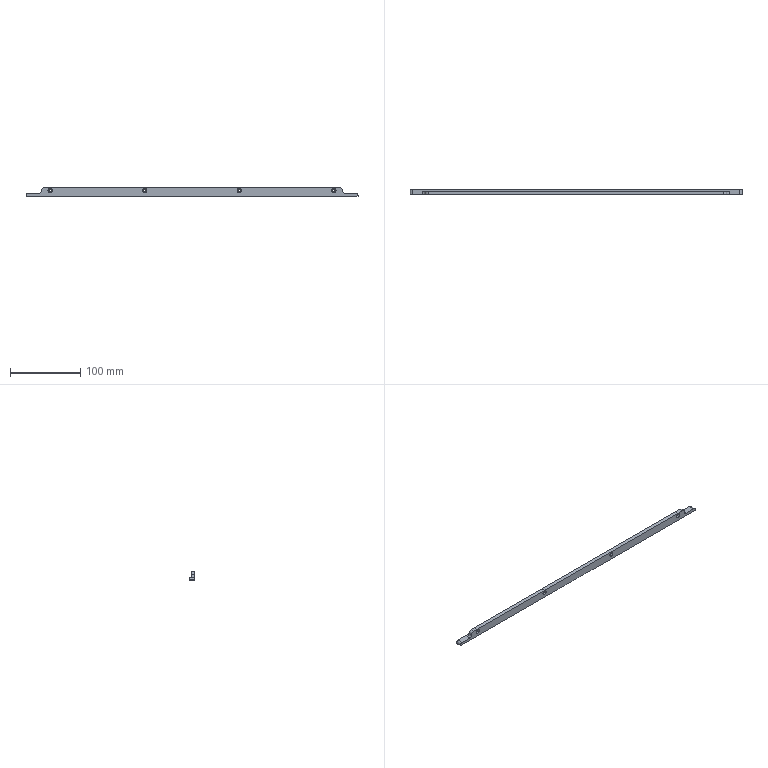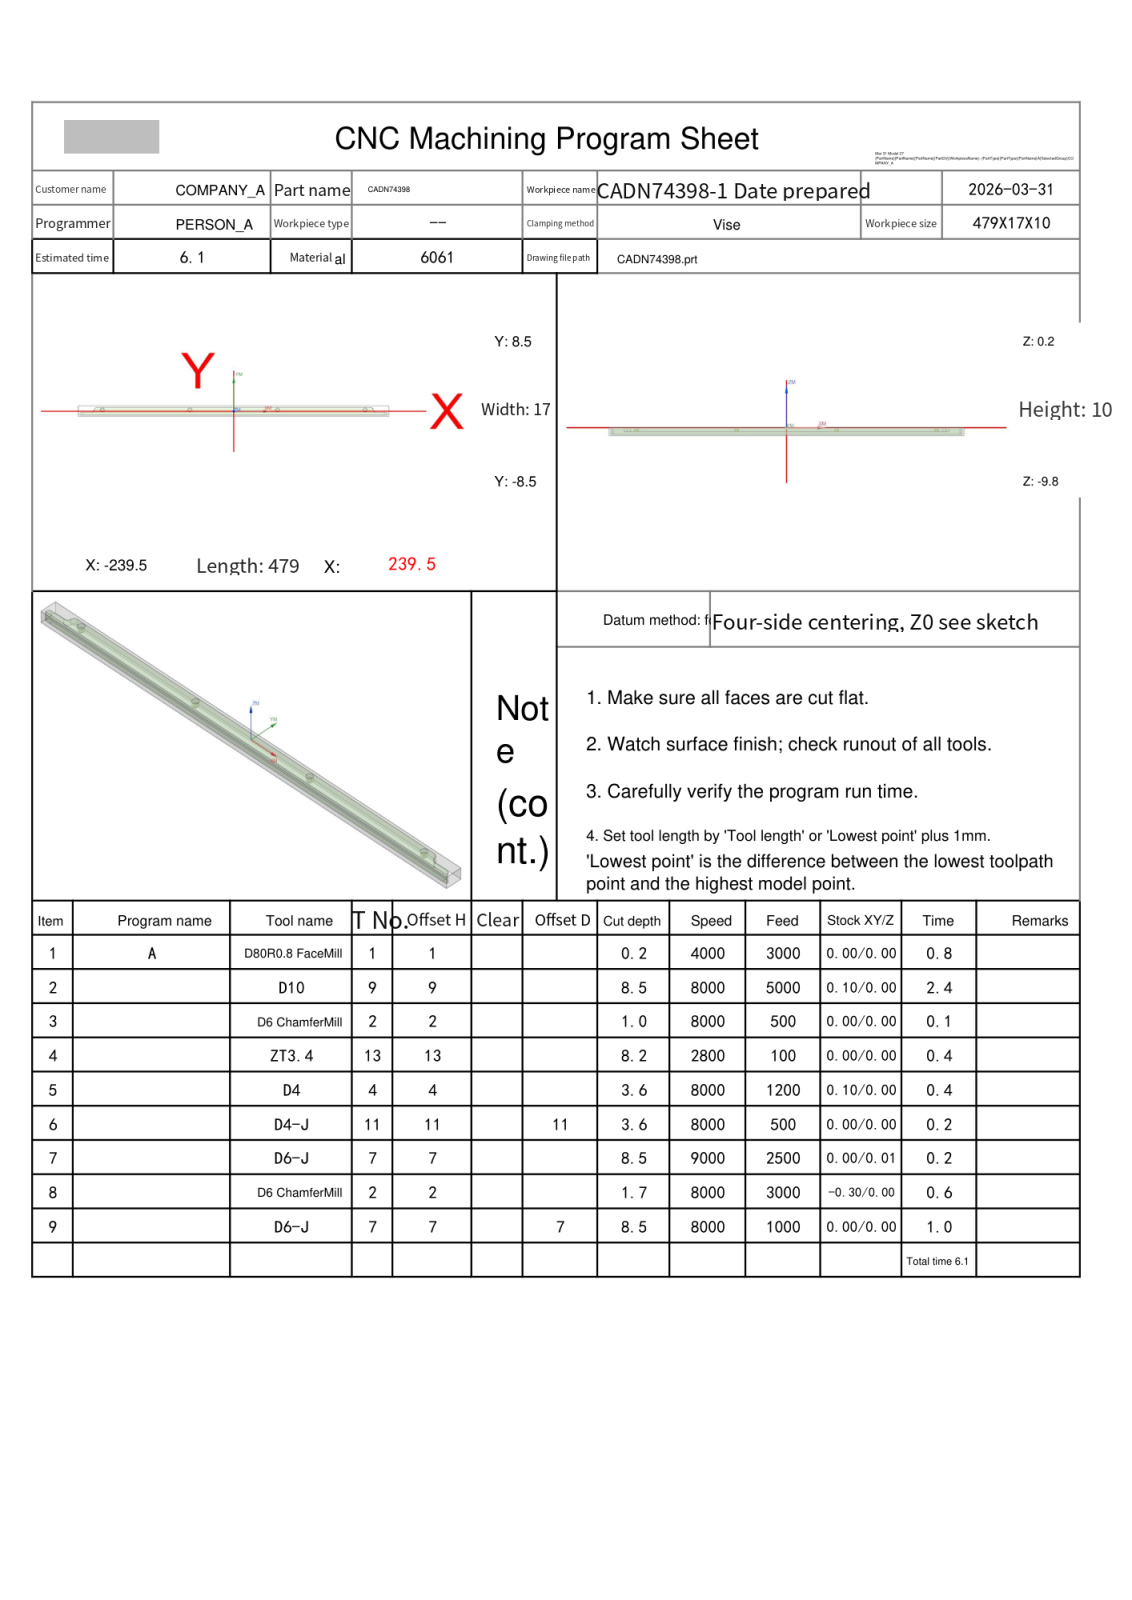NC program | NX | posted by the shop | part box 474 x 8.3 x 12 mm
Lines 1 to 412 of 2396:
%
O0001
(Machine time: 7.99 MIN)
(===Total Tool:7===)
(T1=D80R0.8 FaceMill D=80.  R=0.8  D-  H01 Z=0.    )
(T9=D10     D=10.  R=0.   D-  H09 Z=-8.3  )
(T2=D6 ChamferMill   D=6.   R=0.   D-  H02 Z=-1.5  )
(T13=ZT3.4  D=3.4  DR_a=118 D-  H13 Z=-8.02 )
(T4=D4      D=4.   R=0.   D-  H04 Z=-3.4  )
(T11=D4-J   D=4.   R=0.   D11 H11 Z=-3.4  )
(T7=D6-J    D=6.   R=0.   D-  H07 Z=-8.3  )
G80 G90 G17 G49 G40
G91 G28 Z0
M01
N1 T01 M06
(D80R0.8 FaceMill  D=80. R=0.8 H=01 ce=0.20 di=0.10)
G00 G90 G54 X282. Y0.0 M03 S4000
G43 H01 Z20.
M08
Z2.1
G01 Z.1 F3000.
X277.
X-277.
X-282.
Z2.1
G00 Z20.
G00 G90 X282. Y0.0 M03 S4000
Z20.
Z2.
G01 Z0.0 F1000.
X277.
X-277.
X-282.
Z2.
G00 Z20.
G91 G28 Z0.0
M05
M09
G91 G28 Z0.0
M01
N2 T09 M06
(D10  D=10. R=0. H=09 ce=0.10 di=0.00)
G00 G90 G54 X0.0 Y-11.1 M03 S8000
G43 H09 Z20.
M08
Z.5
G01 X-237. Z.309 F5000.
G02 X-242.1 Y-6. Z.303 I0.0 J5.1
G01 Y-5. Z.302
G02 X-234. Y3.1 Z.292 I8.1 J0.0
G01 X-220.033 Z.28
G02 X-211. Y11.1 Z.27 I9.033 J-1.1
G01 X211. Z-.07
G02 X220.033 Y3.1 Z-.08 I0.0 J-9.1
G01 X234. Z-.092
G02 X242.1 Y-5. Z-.102 I0.0 J-8.1
G01 Y-6. Z-.103
G02 X237. Y-11.1 Z-.109 I-5.1 J0.0
G01 X-237. Z-.491
G02 X-242.1 Y-6. Z-.497 I0.0 J5.1
G01 Y-5. Z-.498
G02 X-234. Y3.1 Z-.508 I8.1 J0.0
G01 X-220.033 Z-.52
G02 X-211. Y11.1 Z-.53 I9.033 J-1.1
G01 X211. Z-.87
G02 X220.033 Y3.1 Z-.88 I0.0 J-9.1
G01 X234. Z-.892
G02 X242.1 Y-5. Z-.902 I0.0 J-8.1
G01 Y-6. Z-.903
G02 X237. Y-11.1 Z-.909 I-5.1 J0.0
G01 X-237. Z-1.291
G02 X-242.1 Y-6. Z-1.297 I0.0 J5.1
G01 Y-5. Z-1.298
G02 X-234. Y3.1 Z-1.308 I8.1 J0.0
G01 X-220.033 Z-1.32
G02 X-211. Y11.1 Z-1.33 I9.033 J-1.1
G01 X211. Z-1.67
G02 X220.033 Y3.1 Z-1.68 I0.0 J-9.1
G01 X234. Z-1.692
G02 X242.1 Y-5. Z-1.702 I0.0 J-8.1
G01 Y-6. Z-1.703
G02 X237. Y-11.1 Z-1.709 I-5.1 J0.0
G01 X-237. Z-2.091
G02 X-242.1 Y-6. Z-2.097 I0.0 J5.1
G01 Y-5. Z-2.098
G02 X-234. Y3.1 Z-2.108 I8.1 J0.0
G01 X-220.033 Z-2.12
G02 X-211. Y11.1 Z-2.13 I9.033 J-1.1
G01 X211. Z-2.47
G02 X220.033 Y3.1 Z-2.48 I0.0 J-9.1
G01 X234. Z-2.492
G02 X242.1 Y-5. Z-2.502 I0.0 J-8.1
G01 Y-6. Z-2.503
G02 X237. Y-11.1 Z-2.509 I-5.1 J0.0
G01 X-237. Z-2.891
G02 X-242.1 Y-6. Z-2.897 I0.0 J5.1
G01 Y-5. Z-2.898
G02 X-234. Y3.1 Z-2.908 I8.1 J0.0
G01 X-220.033 Z-2.92
G02 X-211. Y11.1 Z-2.93 I9.033 J-1.1
G01 X211. Z-3.27
G02 X220.033 Y3.1 Z-3.28 I0.0 J-9.1
G01 X234. Z-3.292
G02 X242.1 Y-5. Z-3.302 I0.0 J-8.1
G01 Y-6. Z-3.303
G02 X237. Y-11.1 Z-3.309 I-5.1 J0.0
G01 X-237. Z-3.691
G02 X-242.1 Y-6. Z-3.697 I0.0 J5.1
G01 Y-5. Z-3.698
G02 X-234. Y3.1 Z-3.708 I8.1 J0.0
G01 X-220.033 Z-3.72
G02 X-211. Y11.1 Z-3.73 I9.033 J-1.1
G01 X211. Z-4.07
G02 X220.033 Y3.1 Z-4.08 I0.0 J-9.1
G01 X234. Z-4.092
G02 X242.1 Y-5. Z-4.102 I0.0 J-8.1
G01 Y-6. Z-4.103
G02 X237. Y-11.1 Z-4.109 I-5.1 J0.0
G01 X-237. Z-4.491
G02 X-242.1 Y-6. Z-4.497 I0.0 J5.1
G01 Y-5. Z-4.498
G02 X-234. Y3.1 Z-4.508 I8.1 J0.0
G01 X-220.033 Z-4.52
G02 X-211. Y11.1 Z-4.53 I9.033 J-1.1
G01 X211. Z-4.87
G02 X220.033 Y3.1 Z-4.88 I0.0 J-9.1
G01 X234. Z-4.892
G02 X242.1 Y-5. Z-4.902 I0.0 J-8.1
G01 Y-6. Z-4.903
G02 X237. Y-11.1 Z-4.909 I-5.1 J0.0
G01 X-237. Z-5.291
G02 X-242.1 Y-6. Z-5.297 I0.0 J5.1
G01 Y-5. Z-5.298
G02 X-234. Y3.1 Z-5.308 I8.1 J0.0
G01 X-220.033 Z-5.32
G02 X-211. Y11.1 Z-5.33 I9.033 J-1.1
G01 X211. Z-5.67
G02 X220.033 Y3.1 Z-5.68 I0.0 J-9.1
G01 X234. Z-5.692
G02 X242.1 Y-5. Z-5.702 I0.0 J-8.1
G01 Y-6. Z-5.703
G02 X237. Y-11.1 Z-5.709 I-5.1 J0.0
G01 X-237. Z-6.091
G02 X-242.1 Y-6. Z-6.097 I0.0 J5.1
G01 Y-5. Z-6.098
G02 X-234. Y3.1 Z-6.108 I8.1 J0.0
G01 X-220.033 Z-6.12
G02 X-211. Y11.1 Z-6.13 I9.033 J-1.1
G01 X211. Z-6.47
G02 X220.033 Y3.1 Z-6.48 I0.0 J-9.1
G01 X234. Z-6.492
G02 X242.1 Y-5. Z-6.502 I0.0 J-8.1
G01 Y-6. Z-6.503
G02 X237. Y-11.1 Z-6.509 I-5.1 J0.0
G01 X-237. Z-6.891
G02 X-242.1 Y-6. Z-6.897 I0.0 J5.1
G01 Y-5. Z-6.898
G02 X-234. Y3.1 Z-6.908 I8.1 J0.0
G01 X-220.033 Z-6.92
G02 X-211. Y11.1 Z-6.93 I9.033 J-1.1
G01 X211. Z-7.27
G02 X220.033 Y3.1 Z-7.28 I0.0 J-9.1
G01 X234. Z-7.292
G02 X242.1 Y-5. Z-7.302 I0.0 J-8.1
G01 Y-6. Z-7.303
G02 X237. Y-11.1 Z-7.309 I-5.1 J0.0
G01 X-237. Z-7.691
G02 X-242.1 Y-6. Z-7.697 I0.0 J5.1
G01 Y-5. Z-7.698
G02 X-234. Y3.1 Z-7.708 I8.1 J0.0
G01 X-220.033 Z-7.72
G02 X-211. Y11.1 Z-7.73 I9.033 J-1.1
G01 X211. Z-8.07
G02 X220.033 Y3.1 Z-8.08 I0.0 J-9.1
G01 X234. Z-8.092
G02 X242.1 Y-5. Z-8.102 I0.0 J-8.1
G01 Y-6. Z-8.103
G02 X237. Y-11.1 Z-8.109 I-5.1 J0.0
G01 X0.0 Z-8.3
X-237.
G02 X-242.1 Y-6. I0.0 J5.1
G01 Y-5.
G02 X-234. Y3.1 I8.1 J0.0
G01 X-220.033
G02 X-211. Y11.1 I9.033 J-1.1
G01 X211.
G02 X220.033 Y3.1 I0.0 J-9.1
G01 X234.
G02 X242.1 Y-5. I0.0 J-8.1
G01 Y-6.
G02 X237. Y-11.1 I-5.1 J0.0
G01 X0.0
X-.5
Z-7.3
G00 Z20.
G91 G28 Z0.0
M05
M09
G91 G28 Z0.0
M01
N3 T02 M06
(D6 ChamferMill  D=6. R=0. H=02 ce=0.00 di=0.00)
G00 G90 G54 X202.5 Y2. M03 S8000
G43 H02 Z20.
M08
G98 G81 X202.5 Y2. Z-.8 R1. F500.
X67.5
X-67.5
X-202.5
G80
G00 Z20.
G91 G28 Z0.0
M05
M09
G91 G28 Z0.0
M01
N4 T13 M06
(ZT3.4 D=3.4 DR_a=118 H=13)
G00 G90 G54 X202.5 Y2. M03 S2800
G43 H13 Z20.
M08
G98 G83 X202.5 Y2. Z-8.021 R1. F100. Q2.
X67.5
X-67.5
X-202.5
G80
G00 Z20.
G91 G28 Z0.0
M05
M09
G91 G28 Z0.0
M01
N5 T04 M06
(D4  D=4. R=0. H=04 ce=0.10 di=0.00)
G00 G90 G54 X202.5 Y2. M03 S8000
G43 H04 Z20.
M08
Z.5
G03 X203.075 Y1.425 I.575 J0.0 F1200.
X203.65 Y2. I0.0 J.575
X203.65 Y2. Z.2 I-1.15 J0.0
X203.65 Y2. Z-.1 I-1.15 J0.0
X203.65 Y2. Z-.4 I-1.15 J0.0
X203.65 Y2. Z-.7 I-1.15 J0.0
X203.65 Y2. Z-1. I-1.15 J0.0
X203.65 Y2. Z-1.3 I-1.15 J0.0
X203.65 Y2. Z-1.6 I-1.15 J0.0
X203.65 Y2. Z-1.9 I-1.15 J0.0
X203.65 Y2. Z-2.2 I-1.15 J0.0
X203.65 Y2. Z-2.5 I-1.15 J0.0
X203.65 Y2. Z-2.8 I-1.15 J0.0
X203.65 Y2. Z-3.1 I-1.15 J0.0
X203.65 Y2. Z-3.4 I-1.15 J0.0
X202.5 Y3.15 I-1.15 J0.0
X201.35 Y2. I0.0 J-1.15
X202.5 Y.85 I1.15 J0.0
X203.65 Y2. I0.0 J1.15
X203.075 Y2.575 I-.575 J0.0
X202.5 Y2. I0.0 J-.575
G00 Z20.
X67.5
Z.5
G03 X68.075 Y1.425 I.575 J0.0
X68.65 Y2. I0.0 J.575
X68.65 Y2. Z.2 I-1.15 J0.0
X68.65 Y2. Z-.1 I-1.15 J0.0
X68.65 Y2. Z-.4 I-1.15 J0.0
X68.65 Y2. Z-.7 I-1.15 J0.0
X68.65 Y2. Z-1. I-1.15 J0.0
X68.65 Y2. Z-1.3 I-1.15 J0.0
X68.65 Y2. Z-1.6 I-1.15 J0.0
X68.65 Y2. Z-1.9 I-1.15 J0.0
X68.65 Y2. Z-2.2 I-1.15 J0.0
X68.65 Y2. Z-2.5 I-1.15 J0.0
X68.65 Y2. Z-2.8 I-1.15 J0.0
X68.65 Y2. Z-3.1 I-1.15 J0.0
X68.65 Y2. Z-3.4 I-1.15 J0.0
X67.5 Y3.15 I-1.15 J0.0
X66.35 Y2. I0.0 J-1.15
X67.5 Y.85 I1.15 J0.0
X68.65 Y2. I0.0 J1.15
X68.075 Y2.575 I-.575 J0.0
X67.5 Y2. I0.0 J-.575
G00 Z20.
X-67.5
Z.5
G03 X-66.925 Y1.425 I.575 J0.0
X-66.35 Y2. I0.0 J.575
X-66.35 Y2. Z.2 I-1.15 J0.0
X-66.35 Y2. Z-.1 I-1.15 J0.0
X-66.35 Y2. Z-.4 I-1.15 J0.0
X-66.35 Y2. Z-.7 I-1.15 J0.0
X-66.35 Y2. Z-1. I-1.15 J0.0
X-66.35 Y2. Z-1.3 I-1.15 J0.0
X-66.35 Y2. Z-1.6 I-1.15 J0.0
X-66.35 Y2. Z-1.9 I-1.15 J0.0
X-66.35 Y2. Z-2.2 I-1.15 J0.0
X-66.35 Y2. Z-2.5 I-1.15 J0.0
X-66.35 Y2. Z-2.8 I-1.15 J0.0
X-66.35 Y2. Z-3.1 I-1.15 J0.0
X-66.35 Y2. Z-3.4 I-1.15 J0.0
X-67.5 Y3.15 I-1.15 J0.0
X-68.65 Y2. I0.0 J-1.15
X-67.5 Y.85 I1.15 J0.0
X-66.35 Y2. I0.0 J1.15
X-66.925 Y2.575 I-.575 J0.0
X-67.5 Y2. I0.0 J-.575
G00 Z20.
X-202.5
Z.5
G03 X-201.925 Y1.425 I.575 J0.0
X-201.35 Y2. I0.0 J.575
X-201.35 Y2. Z.2 I-1.15 J0.0
X-201.35 Y2. Z-.1 I-1.15 J0.0
X-201.35 Y2. Z-.4 I-1.15 J0.0
X-201.35 Y2. Z-.7 I-1.15 J0.0
X-201.35 Y2. Z-1. I-1.15 J0.0
X-201.35 Y2. Z-1.3 I-1.15 J0.0
X-201.35 Y2. Z-1.6 I-1.15 J0.0
X-201.35 Y2. Z-1.9 I-1.15 J0.0
X-201.35 Y2. Z-2.2 I-1.15 J0.0
X-201.35 Y2. Z-2.5 I-1.15 J0.0
X-201.35 Y2. Z-2.8 I-1.15 J0.0
X-201.35 Y2. Z-3.1 I-1.15 J0.0
X-201.35 Y2. Z-3.4 I-1.15 J0.0
X-202.5 Y3.15 I-1.15 J0.0
X-203.65 Y2. I0.0 J-1.15
X-202.5 Y.85 I1.15 J0.0
X-201.35 Y2. I0.0 J1.15
X-201.925 Y2.575 I-.575 J0.0
X-202.5 Y2. I0.0 J-.575
G00 Z20.
G91 G28 Z0.0
M05
M09
G91 G28 Z0.0
M01
N6 T11 M06
(D4-J  D=4. R=0. H=11 ce=0.00 di=0.00)
G00 G90 G54 X202.5 Y2. M03 S8000
G43 H11 Z20.
M08
Z.5
G41 D11
G01 X202.562 Y1.81 F500.
G03 X203.141 Y1.391 I.579 J.19
X203.75 Y2. I0.0 J.609
X202.734 Y.772 Z-3.4 I-1.25 J0.0
X203.75 Y2. I-.234 J1.228
X202.5 Y3.25 I-1.25 J0.0
X201.25 Y2. I0.0 J-1.25
X202.5 Y.75 I1.25 J0.0
X202.734 Y.772 I0.0 J1.25
X203.229 Y1.37 I-.114 J.598
X202.698 Y1.974 I-.609 J0.0
G01 G40 X202.5 Y2.
G00 Z20.
X67.5
Z.5
G41 D11
G01 X67.562 Y1.81
G03 X68.141 Y1.391 I.579 J.19
X68.75 Y2. I0.0 J.609
X67.734 Y.772 Z-3.4 I-1.25 J0.0
X68.75 Y2. I-.234 J1.228
X67.5 Y3.25 I-1.25 J0.0
X66.25 Y2. I0.0 J-1.25
X67.5 Y.75 I1.25 J0.0
X67.734 Y.772 I0.0 J1.25
X68.229 Y1.37 I-.114 J.598
X67.698 Y1.974 I-.609 J0.0
G01 G40 X67.5 Y2.
G00 Z20.
X-67.5
Z.5
G41 D11
G01 X-67.438 Y1.81
G03 X-66.859 Y1.391 I.579 J.19
X-66.25 Y2. I0.0 J.609
X-67.266 Y.772 Z-3.4 I-1.25 J0.0
X-66.25 Y2. I-.234 J1.228
X-67.5 Y3.25 I-1.25 J0.0
X-68.75 Y2. I0.0 J-1.25
X-67.5 Y.75 I1.25 J0.0
X-67.266 Y.772 I0.0 J1.25
X-66.771 Y1.37 I-.114 J.598
X-67.302 Y1.974 I-.609 J0.0
G01 G40 X-67.5 Y2.
G00 Z20.
X-202.5
Z.5
G41 D11
G01 X-202.438 Y1.81
G03 X-201.859 Y1.391 I.579 J.19
X-201.25 Y2. I0.0 J.609
X-202.266 Y.772 Z-3.4 I-1.25 J0.0
X-201.25 Y2. I-.234 J1.228
X-202.5 Y3.25 I-1.25 J0.0
X-203.75 Y2. I0.0 J-1.25
X-202.5 Y.75 I1.25 J0.0
X-202.266 Y.772 I0.0 J1.25
X-201.771 Y1.37 I-.114 J.598
X-202.302 Y1.974 I-.609 J0.0
G01 G40 X-202.5 Y2.
G00 Z20.
G91 G28 Z0.0
M05
M09
G91 G28 Z0.0
M01